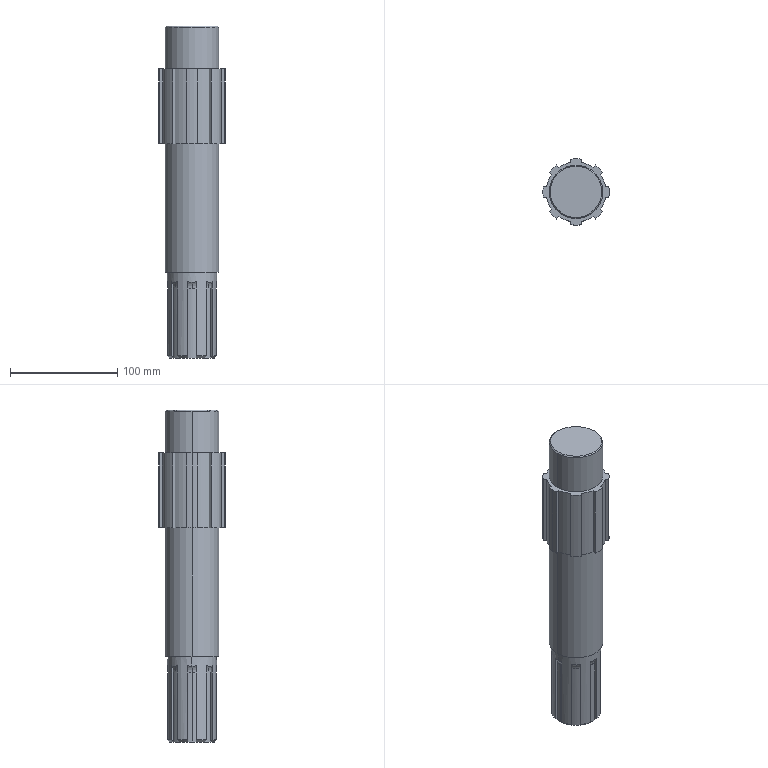Part | SolidWorks | features ICE 4, Chamfer 2, CirPattern 1, Extrusion 1, SweepCut 1 | 1 solid | 95 faces | box 62 x 62 x 310 mm | volume 627287 mm3 | plane 37 | cylinder 32 | torus 16 | cone 10 | commonest cylinder face diameters 42 x9 62 x9 56 x8 50 x4 46 x2